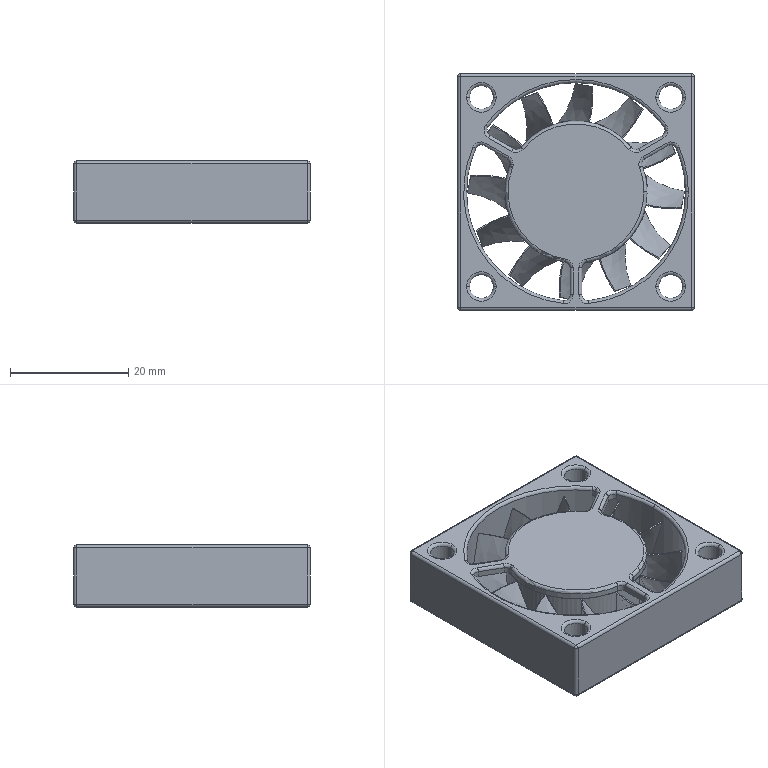Part | SolidWorks | 13 solids | 375 faces | box 40 x 40 x 10.5 mm | volume 24242 mm3 | cylinder 172 | plane 91 | spline 72 | torus 32 | sphere 8 | commonest cylinder face diameters 24 x28 5 x26 8 x24 21 x24 1 x18 2 x14